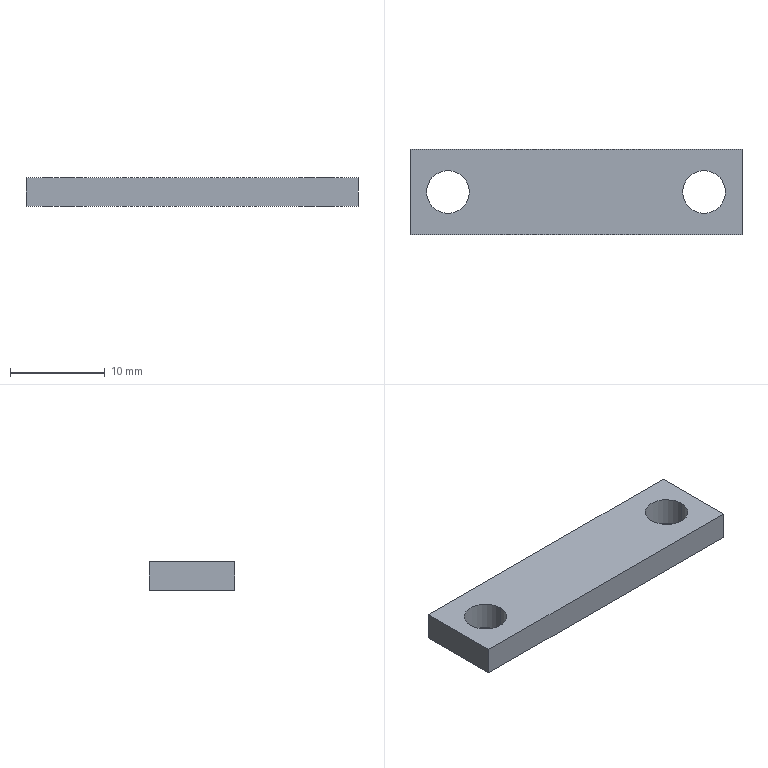Part | SolidWorks | features Extrusion 1 | 1 solid | 10 faces | box 35 x 9 x 3 mm | volume 849.574 mm3 | plane 6 | cylinder 4 | commonest cylinder face diameters 4.5 x4
STEP:
#1=CARTESIAN_POINT('',(11.25,0.,1.5));
#2=VERTEX_POINT('',#1);
#3=CARTESIAN_POINT('',(15.75,0.,1.5));
#4=VERTEX_POINT('',#3);
#5=CARTESIAN_POINT('',(13.5,0.,1.5));
#6=DIRECTION('',(0.,0.,1.));
#7=DIRECTION('',(1.,0.,0.));
#8=AXIS2_PLACEMENT_3D('',#5,#6,#7);
#9=CIRCLE('',#8,2.25);
#10=EDGE_CURVE('',#2,#4,#9,.T.);
#11=ORIENTED_EDGE('',*,*,#10,.T.);
#12=CARTESIAN_POINT('',(15.75,0.,-1.5));
#13=VERTEX_POINT('',#12);
#14=CARTESIAN_POINT('',(15.75,0.,1.5));
#15=DIRECTION('',(0.,0.,-1.));
#16=VECTOR('',#15,1000.);
#17=LINE('',#14,#16);
#18=EDGE_CURVE('',#4,#13,#17,.T.);
#19=ORIENTED_EDGE('',*,*,#18,.T.);
#20=CARTESIAN_POINT('',(11.25,0.,-1.5));
#21=VERTEX_POINT('',#20);
#22=CARTESIAN_POINT('',(13.5,0.,-1.5));
#23=DIRECTION('',(0.,0.,1.));
#24=DIRECTION('',(1.,0.,0.));
#25=AXIS2_PLACEMENT_3D('',#22,#23,#24);
#26=CIRCLE('',#25,2.25);
#27=EDGE_CURVE('',#21,#13,#26,.T.);
#28=ORIENTED_EDGE('',*,*,#27,.F.);
#29=CARTESIAN_POINT('',(11.25,0.,1.5));
#30=DIRECTION('',(0.,0.,-1.));
#31=VECTOR('',#30,1000.);
#32=LINE('',#29,#31);
#33=EDGE_CURVE('',#2,#21,#32,.T.);
#34=ORIENTED_EDGE('',*,*,#33,.F.);
#35=EDGE_LOOP('',(#11,#19,#28,#34));
#36=FACE_OUTER_BOUND('',#35,.T.);
#37=CARTESIAN_POINT('',(13.5,0.,1.5));
#38=DIRECTION('',(0.,0.,-1.));
#39=DIRECTION('',(-1.,0.,0.));
#40=AXIS2_PLACEMENT_3D('',#37,#38,#39);
#41=CYLINDRICAL_SURFACE('',#40,2.25);
#42=ADVANCED_FACE('',(#36),#41,.F.);
#43=CARTESIAN_POINT('',(-15.75,0.,1.5));
#44=VERTEX_POINT('',#43);
#45=CARTESIAN_POINT('',(-11.25,0.,1.5));
#46=VERTEX_POINT('',#45);
#47=CARTESIAN_POINT('',(-13.5,0.,1.5));
#48=DIRECTION('',(0.,0.,1.));
#49=DIRECTION('',(1.,0.,0.));
#50=AXIS2_PLACEMENT_3D('',#47,#48,#49);
#51=CIRCLE('',#50,2.25);
#52=EDGE_CURVE('',#44,#46,#51,.T.);
#53=ORIENTED_EDGE('',*,*,#52,.T.);
#54=CARTESIAN_POINT('',(-11.25,0.,-1.5));
#55=VERTEX_POINT('',#54);
#56=CARTESIAN_POINT('',(-11.25,0.,1.5));
#57=DIRECTION('',(0.,0.,-1.));
#58=VECTOR('',#57,1000.);
#59=LINE('',#56,#58);
#60=EDGE_CURVE('',#46,#55,#59,.T.);
#61=ORIENTED_EDGE('',*,*,#60,.T.);
#62=CARTESIAN_POINT('',(-15.75,0.,-1.5));
#63=VERTEX_POINT('',#62);
#64=CARTESIAN_POINT('',(-13.5,0.,-1.5));
#65=DIRECTION('',(0.,0.,1.));
#66=DIRECTION('',(1.,0.,0.));
#67=AXIS2_PLACEMENT_3D('',#64,#65,#66);
#68=CIRCLE('',#67,2.25);
#69=EDGE_CURVE('',#63,#55,#68,.T.);
#70=ORIENTED_EDGE('',*,*,#69,.F.);
#71=CARTESIAN_POINT('',(-15.75,0.,1.5));
#72=DIRECTION('',(0.,0.,-1.));
#73=VECTOR('',#72,1000.);
#74=LINE('',#71,#73);
#75=EDGE_CURVE('',#44,#63,#74,.T.);
#76=ORIENTED_EDGE('',*,*,#75,.F.);
#77=EDGE_LOOP('',(#53,#61,#70,#76));
#78=FACE_OUTER_BOUND('',#77,.T.);
#79=CARTESIAN_POINT('',(-13.5,0.,1.5));
#80=DIRECTION('',(0.,0.,-1.));
#81=DIRECTION('',(-1.,0.,0.));
#82=AXIS2_PLACEMENT_3D('',#79,#80,#81);
#83=CYLINDRICAL_SURFACE('',#82,2.25);
#84=ADVANCED_FACE('',(#78),#83,.F.);
#85=CARTESIAN_POINT('',(17.5,-4.5,1.5));
#86=VERTEX_POINT('',#85);
#87=CARTESIAN_POINT('',(17.5,4.5,1.5));
#88=VERTEX_POINT('',#87);
#89=CARTESIAN_POINT('',(17.5,-4.5,1.5));
#90=DIRECTION('',(0.,1.,0.));
#91=VECTOR('',#90,1000.);
#92=LINE('',#89,#91);
#93=EDGE_CURVE('',#86,#88,#92,.T.);
#94=ORIENTED_EDGE('',*,*,#93,.T.);
#95=CARTESIAN_POINT('',(-17.5,4.5,1.5));
#96=VERTEX_POINT('',#95);
#97=CARTESIAN_POINT('',(-17.5,4.5,1.5));
#98=DIRECTION('',(-1.,0.,0.));
#99=VECTOR('',#98,1000.);
#100=LINE('',#97,#99);
#101=EDGE_CURVE('',#88,#96,#100,.T.);
#102=ORIENTED_EDGE('',*,*,#101,.T.);
#103=CARTESIAN_POINT('',(-17.5,-4.5,1.5));
#104=VERTEX_POINT('',#103);
#105=CARTESIAN_POINT('',(-17.5,-4.5,1.5));
#106=DIRECTION('',(0.,-1.,0.));
#107=VECTOR('',#106,1000.);
#108=LINE('',#105,#107);
#109=EDGE_CURVE('',#96,#104,#108,.T.);
#110=ORIENTED_EDGE('',*,*,#109,.T.);
#111=CARTESIAN_POINT('',(-17.5,-4.5,1.5));
#112=DIRECTION('',(1.,0.,0.));
#113=VECTOR('',#112,1000.);
#114=LINE('',#111,#113);
#115=EDGE_CURVE('',#104,#86,#114,.T.);
#116=ORIENTED_EDGE('',*,*,#115,.T.);
#117=EDGE_LOOP('',(#94,#102,#110,#116));
#118=FACE_OUTER_BOUND('',#117,.T.);
#119=ORIENTED_EDGE('',*,*,#52,.F.);
#120=CARTESIAN_POINT('',(-13.5,0.,1.5));
#121=DIRECTION('',(0.,0.,1.));
#122=DIRECTION('',(1.,0.,0.));
#123=AXIS2_PLACEMENT_3D('',#120,#121,#122);
#124=CIRCLE('',#123,2.25);
#125=EDGE_CURVE('',#46,#44,#124,.T.);
#126=ORIENTED_EDGE('',*,*,#125,.F.);
#127=EDGE_LOOP('',(#119,#126));
#128=FACE_BOUND('',#127,.T.);
#129=ORIENTED_EDGE('',*,*,#10,.F.);
#130=CARTESIAN_POINT('',(13.5,0.,1.5));
#131=DIRECTION('',(0.,0.,1.));
#132=DIRECTION('',(1.,0.,0.));
#133=AXIS2_PLACEMENT_3D('',#130,#131,#132);
#134=CIRCLE('',#133,2.25);
#135=EDGE_CURVE('',#4,#2,#134,.T.);
#136=ORIENTED_EDGE('',*,*,#135,.F.);
#137=EDGE_LOOP('',(#129,#136));
#138=FACE_BOUND('',#137,.T.);
#139=CARTESIAN_POINT('',(0.,0.,1.5));
#140=DIRECTION('',(0.,0.,-1.));
#141=DIRECTION('',(-1.,0.,0.));
#142=AXIS2_PLACEMENT_3D('',#139,#140,#141);
#143=PLANE('',#142);
#144=ADVANCED_FACE('',(#118,#128,#138),#143,.F.);
#145=ORIENTED_EDGE('',*,*,#69,.T.);
#146=CARTESIAN_POINT('',(-13.5,0.,-1.5));
#147=DIRECTION('',(0.,0.,1.));
#148=DIRECTION('',(1.,0.,0.));
#149=AXIS2_PLACEMENT_3D('',#146,#147,#148);
#150=CIRCLE('',#149,2.25);
#151=EDGE_CURVE('',#55,#63,#150,.T.);
#152=ORIENTED_EDGE('',*,*,#151,.T.);
#153=EDGE_LOOP('',(#145,#152));
#154=FACE_BOUND('',#153,.T.);
#155=CARTESIAN_POINT('',(17.5,-4.5,-1.5));
#156=VERTEX_POINT('',#155);
#157=CARTESIAN_POINT('',(17.5,4.5,-1.5));
#158=VERTEX_POINT('',#157);
#159=CARTESIAN_POINT('',(17.5,-4.5,-1.5));
#160=DIRECTION('',(0.,1.,0.));
#161=VECTOR('',#160,1000.);
#162=LINE('',#159,#161);
#163=EDGE_CURVE('',#156,#158,#162,.T.);
#164=ORIENTED_EDGE('',*,*,#163,.F.);
#165=CARTESIAN_POINT('',(-17.5,-4.5,-1.5));
#166=VERTEX_POINT('',#165);
#167=CARTESIAN_POINT('',(-17.5,-4.5,-1.5));
#168=DIRECTION('',(1.,0.,0.));
#169=VECTOR('',#168,1000.);
#170=LINE('',#167,#169);
#171=EDGE_CURVE('',#166,#156,#170,.T.);
#172=ORIENTED_EDGE('',*,*,#171,.F.);
#173=CARTESIAN_POINT('',(-17.5,4.5,-1.5));
#174=VERTEX_POINT('',#173);
#175=CARTESIAN_POINT('',(-17.5,-4.5,-1.5));
#176=DIRECTION('',(0.,-1.,0.));
#177=VECTOR('',#176,1000.);
#178=LINE('',#175,#177);
#179=EDGE_CURVE('',#174,#166,#178,.T.);
#180=ORIENTED_EDGE('',*,*,#179,.F.);
#181=CARTESIAN_POINT('',(-17.5,4.5,-1.5));
#182=DIRECTION('',(-1.,0.,0.));
#183=VECTOR('',#182,1000.);
#184=LINE('',#181,#183);
#185=EDGE_CURVE('',#158,#174,#184,.T.);
#186=ORIENTED_EDGE('',*,*,#185,.F.);
#187=EDGE_LOOP('',(#164,#172,#180,#186));
#188=FACE_OUTER_BOUND('',#187,.T.);
#189=ORIENTED_EDGE('',*,*,#27,.T.);
#190=CARTESIAN_POINT('',(13.5,0.,-1.5));
#191=DIRECTION('',(0.,0.,1.));
#192=DIRECTION('',(1.,0.,0.));
#193=AXIS2_PLACEMENT_3D('',#190,#191,#192);
#194=CIRCLE('',#193,2.25);
#195=EDGE_CURVE('',#13,#21,#194,.T.);
#196=ORIENTED_EDGE('',*,*,#195,.T.);
#197=EDGE_LOOP('',(#189,#196));
#198=FACE_BOUND('',#197,.T.);
#199=CARTESIAN_POINT('',(0.,0.,-1.5));
#200=DIRECTION('',(0.,0.,-1.));
#201=DIRECTION('',(-1.,0.,0.));
#202=AXIS2_PLACEMENT_3D('',#199,#200,#201);
#203=PLANE('',#202);
#204=ADVANCED_FACE('',(#154,#188,#198),#203,.T.);
#205=ORIENTED_EDGE('',*,*,#163,.T.);
#206=CARTESIAN_POINT('',(17.5,4.5,1.5));
#207=DIRECTION('',(0.,0.,-1.));
#208=VECTOR('',#207,1000.);
#209=LINE('',#206,#208);
#210=EDGE_CURVE('',#88,#158,#209,.T.);
#211=ORIENTED_EDGE('',*,*,#210,.F.);
#212=ORIENTED_EDGE('',*,*,#93,.F.);
#213=CARTESIAN_POINT('',(17.5,-4.5,1.5));
#214=DIRECTION('',(0.,0.,-1.));
#215=VECTOR('',#214,1000.);
#216=LINE('',#213,#215);
#217=EDGE_CURVE('',#86,#156,#216,.T.);
#218=ORIENTED_EDGE('',*,*,#217,.T.);
#219=EDGE_LOOP('',(#205,#211,#212,#218));
#220=FACE_OUTER_BOUND('',#219,.T.);
#221=CARTESIAN_POINT('',(17.5,-4.5,1.5));
#222=DIRECTION('',(-1.,0.,0.));
#223=DIRECTION('',(0.,0.,1.));
#224=AXIS2_PLACEMENT_3D('',#221,#222,#223);
#225=PLANE('',#224);
#226=ADVANCED_FACE('',(#220),#225,.F.);
#227=ORIENTED_EDGE('',*,*,#185,.T.);
#228=CARTESIAN_POINT('',(-17.5,4.5,1.5));
#229=DIRECTION('',(0.,0.,-1.));
#230=VECTOR('',#229,1000.);
#231=LINE('',#228,#230);
#232=EDGE_CURVE('',#96,#174,#231,.T.);
#233=ORIENTED_EDGE('',*,*,#232,.F.);
#234=ORIENTED_EDGE('',*,*,#101,.F.);
#235=ORIENTED_EDGE('',*,*,#210,.T.);
#236=EDGE_LOOP('',(#227,#233,#234,#235));
#237=FACE_OUTER_BOUND('',#236,.T.);
#238=CARTESIAN_POINT('',(-17.5,4.5,1.5));
#239=DIRECTION('',(0.,-1.,0.));
#240=DIRECTION('',(0.,0.,-1.));
#241=AXIS2_PLACEMENT_3D('',#238,#239,#240);
#242=PLANE('',#241);
#243=ADVANCED_FACE('',(#237),#242,.F.);
#244=ORIENTED_EDGE('',*,*,#179,.T.);
#245=CARTESIAN_POINT('',(-17.5,-4.5,1.5));
#246=DIRECTION('',(0.,0.,-1.));
#247=VECTOR('',#246,1000.);
#248=LINE('',#245,#247);
#249=EDGE_CURVE('',#104,#166,#248,.T.);
#250=ORIENTED_EDGE('',*,*,#249,.F.);
#251=ORIENTED_EDGE('',*,*,#109,.F.);
#252=ORIENTED_EDGE('',*,*,#232,.T.);
#253=EDGE_LOOP('',(#244,#250,#251,#252));
#254=FACE_OUTER_BOUND('',#253,.T.);
#255=CARTESIAN_POINT('',(-17.5,-4.5,1.5));
#256=DIRECTION('',(1.,0.,0.));
#257=DIRECTION('',(0.,0.,-1.));
#258=AXIS2_PLACEMENT_3D('',#255,#256,#257);
#259=PLANE('',#258);
#260=ADVANCED_FACE('',(#254),#259,.F.);
#261=ORIENTED_EDGE('',*,*,#171,.T.);
#262=ORIENTED_EDGE('',*,*,#217,.F.);
#263=ORIENTED_EDGE('',*,*,#115,.F.);
#264=ORIENTED_EDGE('',*,*,#249,.T.);
#265=EDGE_LOOP('',(#261,#262,#263,#264));
#266=FACE_OUTER_BOUND('',#265,.T.);
#267=CARTESIAN_POINT('',(-17.5,-4.5,1.5));
#268=DIRECTION('',(0.,1.,0.));
#269=DIRECTION('',(0.,0.,1.));
#270=AXIS2_PLACEMENT_3D('',#267,#268,#269);
#271=PLANE('',#270);
#272=ADVANCED_FACE('',(#266),#271,.F.);
#273=ORIENTED_EDGE('',*,*,#60,.F.);
#274=ORIENTED_EDGE('',*,*,#125,.T.);
#275=ORIENTED_EDGE('',*,*,#75,.T.);
#276=ORIENTED_EDGE('',*,*,#151,.F.);
#277=EDGE_LOOP('',(#273,#274,#275,#276));
#278=FACE_OUTER_BOUND('',#277,.T.);
#279=CARTESIAN_POINT('',(-13.5,0.,1.5));
#280=DIRECTION('',(0.,0.,-1.));
#281=DIRECTION('',(-1.,0.,0.));
#282=AXIS2_PLACEMENT_3D('',#279,#280,#281);
#283=CYLINDRICAL_SURFACE('',#282,2.25);
#284=ADVANCED_FACE('',(#278),#283,.F.);
#285=ORIENTED_EDGE('',*,*,#18,.F.);
#286=ORIENTED_EDGE('',*,*,#135,.T.);
#287=ORIENTED_EDGE('',*,*,#33,.T.);
#288=ORIENTED_EDGE('',*,*,#195,.F.);
#289=EDGE_LOOP('',(#285,#286,#287,#288));
#290=FACE_OUTER_BOUND('',#289,.T.);
#291=CARTESIAN_POINT('',(13.5,0.,1.5));
#292=DIRECTION('',(0.,0.,-1.));
#293=DIRECTION('',(-1.,0.,0.));
#294=AXIS2_PLACEMENT_3D('',#291,#292,#293);
#295=CYLINDRICAL_SURFACE('',#294,2.25);
#296=ADVANCED_FACE('',(#290),#295,.F.);
#297=CLOSED_SHELL('',(#42,#84,#144,#204,#226,#243,#260,#272,#284,#296));
#298=MANIFOLD_SOLID_BREP('',#297);
#299=CARTESIAN_POINT('',(0.,0.,0.));
#300=DIRECTION('',(0.,0.,1.));
#301=DIRECTION('',(1.,0.,0.));
#302=AXIS2_PLACEMENT_3D('',#299,#300,#301);
#303=(LENGTH_UNIT()NAMED_UNIT(*)SI_UNIT(.MILLI.,.METRE.));
#304=UNCERTAINTY_MEASURE_WITH_UNIT(LENGTH_MEASURE(0.00001),#303,'','');
#305=(NAMED_UNIT(*)PLANE_ANGLE_UNIT()SI_UNIT($,.RADIAN.));
#306=(NAMED_UNIT(*)SI_UNIT($,.STERADIAN.)SOLID_ANGLE_UNIT());
#307=(GEOMETRIC_REPRESENTATION_CONTEXT(3)GLOBAL_UNCERTAINTY_ASSIGNED_CONTEXT((#304))GLOBAL_UNIT_ASSIGNED_CONTEXT((#303,#305,#306))REPRESENTATION_CONTEXT('',''));
#308=ADVANCED_BREP_SHAPE_REPRESENTATION('',(#298,#302),#307);